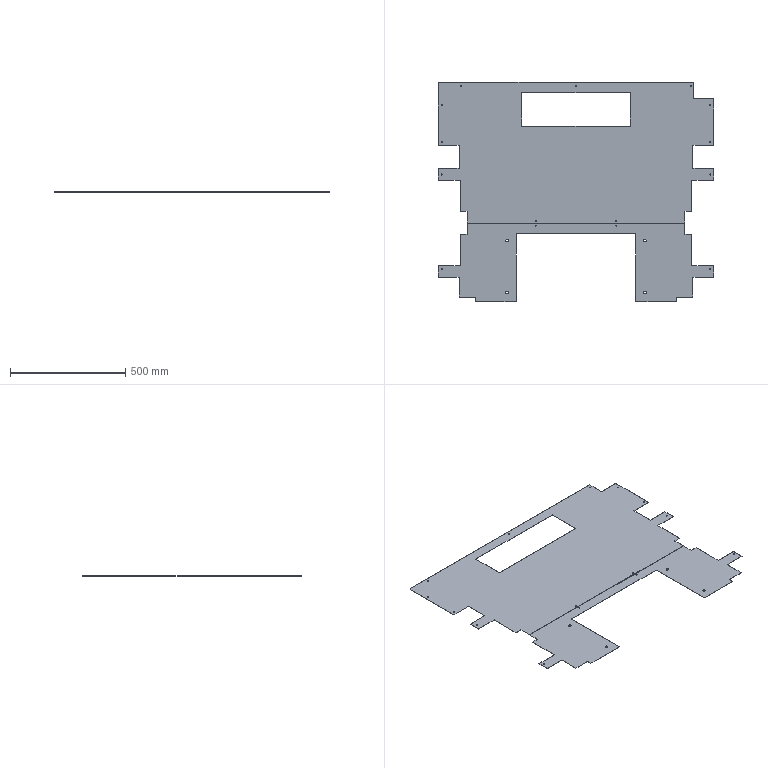Part | SolidWorks | features ICE 11, Cut 5, Fillet 2, Extrusion 1 | 2 solids | 94 faces | box 1195 x 952 x 0.8 mm | volume 633597 mm3 | plane 54 | cylinder 40 | commonest cylinder face diameters 4.5 x30 11 x8 10 x1 13 x1